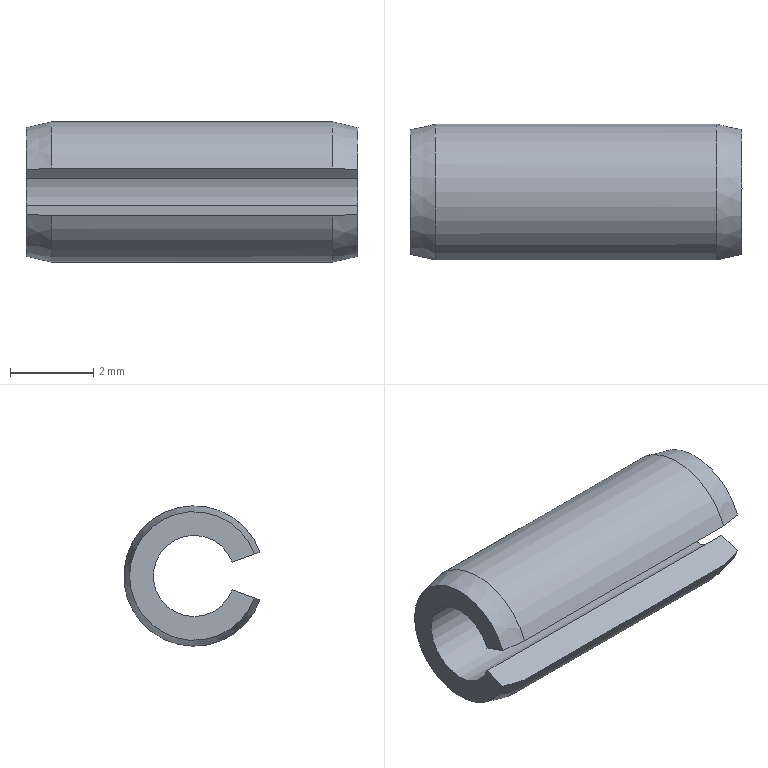Part | NX | features solid 2 | 1 solid | 8 faces | box 7.995 x 3.276 x 3.378 mm | volume 41.565 mm3 | plane 4 | cylinder 2 | cone 2 | commonest cylinder face diameters 1.956 x1 3.378 x1
STEP:
#1=CARTESIAN_POINT('',(282.619,2079.482,26.517));
#2=VERTEX_POINT('',#1);
#3=CARTESIAN_POINT('',(282.619,2079.482,27.673));
#4=VERTEX_POINT('',#3);
#5=CARTESIAN_POINT('',(282.619,2081.069,27.095));
#6=DIRECTION('',(1.,0.,-0.000000164));
#7=DIRECTION('',(-0.000000056,-0.9397,-0.342));
#8=AXIS2_PLACEMENT_3D('',#5,#6,#7);
#9=CIRCLE('',#8,1.689);
#10=EDGE_CURVE('',#2,#4,#9,.T.);
#11=ORIENTED_EDGE('',*,*,#10,.T.);
#12=CARTESIAN_POINT('',(289.395,2079.482,27.673));
#13=VERTEX_POINT('',#12);
#14=CARTESIAN_POINT('',(282.619,2079.482,27.673));
#15=DIRECTION('',(1.,0.,-0.000000164));
#16=VECTOR('',#15,1000.);
#17=LINE('',#14,#16);
#18=EDGE_CURVE('',#4,#13,#17,.T.);
#19=ORIENTED_EDGE('',*,*,#18,.T.);
#20=CARTESIAN_POINT('',(289.395,2081.069,25.406));
#21=VERTEX_POINT('',#20);
#22=CARTESIAN_POINT('',(289.395,2081.069,27.095));
#23=DIRECTION('',(1.,0.,-0.000000164));
#24=DIRECTION('',(-0.000000164,0.,-1.));
#25=AXIS2_PLACEMENT_3D('',#22,#23,#24);
#26=CIRCLE('',#25,1.689);
#27=EDGE_CURVE('',#21,#13,#26,.T.);
#28=ORIENTED_EDGE('',*,*,#27,.F.);
#29=CARTESIAN_POINT('',(289.395,2079.482,26.517));
#30=VERTEX_POINT('',#29);
#31=CARTESIAN_POINT('',(289.395,2081.069,27.095));
#32=DIRECTION('',(1.,0.,-0.000000164));
#33=DIRECTION('',(-0.000000056,-0.9397,-0.342));
#34=AXIS2_PLACEMENT_3D('',#31,#32,#33);
#35=CIRCLE('',#34,1.689);
#36=EDGE_CURVE('',#30,#21,#35,.T.);
#37=ORIENTED_EDGE('',*,*,#36,.F.);
#38=CARTESIAN_POINT('',(289.395,2079.482,26.517));
#39=DIRECTION('',(-1.,0.,0.000000164));
#40=VECTOR('',#39,1000.);
#41=LINE('',#38,#40);
#42=EDGE_CURVE('',#30,#2,#41,.T.);
#43=ORIENTED_EDGE('',*,*,#42,.T.);
#44=EDGE_LOOP('',(#11,#19,#28,#37,#43));
#45=FACE_BOUND('',#44,.T.);
#46=CARTESIAN_POINT('',(288.284,2081.069,27.095));
#47=DIRECTION('',(-1.,0.,0.000000164));
#48=DIRECTION('',(0.000000164,0.,1.));
#49=AXIS2_PLACEMENT_3D('',#46,#47,#48);
#50=CYLINDRICAL_SURFACE('',#49,1.689);
#51=ADVANCED_FACE('',(#45),#50,.T.);
#52=CARTESIAN_POINT('',(282.009,2079.613,26.565));
#53=VERTEX_POINT('',#52);
#54=CARTESIAN_POINT('',(282.009,2079.613,26.565));
#55=DIRECTION('',(0.9747,-0.2099,-0.0764));
#56=VECTOR('',#55,1000.);
#57=LINE('',#54,#56);
#58=EDGE_CURVE('',#53,#2,#57,.T.);
#59=ORIENTED_EDGE('',*,*,#58,.T.);
#60=ORIENTED_EDGE('',*,*,#42,.F.);
#61=CARTESIAN_POINT('',(290.004,2079.613,26.565));
#62=VERTEX_POINT('',#61);
#63=CARTESIAN_POINT('',(289.395,2079.482,26.517));
#64=DIRECTION('',(0.9747,0.2099,0.0764));
#65=VECTOR('',#64,1000.);
#66=LINE('',#63,#65);
#67=EDGE_CURVE('',#30,#62,#66,.T.);
#68=ORIENTED_EDGE('',*,*,#67,.T.);
#69=CARTESIAN_POINT('',(290.004,2080.15,26.761));
#70=VERTEX_POINT('',#69);
#71=CARTESIAN_POINT('',(290.004,2080.15,26.761));
#72=DIRECTION('',(-0.000000056,-0.9397,-0.342));
#73=VECTOR('',#72,1000.);
#74=LINE('',#71,#73);
#75=EDGE_CURVE('',#70,#62,#74,.T.);
#76=ORIENTED_EDGE('',*,*,#75,.F.);
#77=CARTESIAN_POINT('',(282.009,2080.15,26.761));
#78=VERTEX_POINT('',#77);
#79=CARTESIAN_POINT('',(282.009,2080.15,26.761));
#80=DIRECTION('',(1.,0.,-0.000000164));
#81=VECTOR('',#80,1000.);
#82=LINE('',#79,#81);
#83=EDGE_CURVE('',#78,#70,#82,.T.);
#84=ORIENTED_EDGE('',*,*,#83,.F.);
#85=CARTESIAN_POINT('',(282.009,2079.613,26.565));
#86=DIRECTION('',(0.000000056,0.9397,0.342));
#87=VECTOR('',#86,1000.);
#88=LINE('',#85,#87);
#89=EDGE_CURVE('',#53,#78,#88,.T.);
#90=ORIENTED_EDGE('',*,*,#89,.F.);
#91=EDGE_LOOP('',(#59,#60,#68,#76,#84,#90));
#92=FACE_BOUND('',#91,.T.);
#93=CARTESIAN_POINT('',(288.284,2080.15,26.761));
#94=DIRECTION('',(-0.000000154,0.342,-0.9397));
#95=DIRECTION('',(0.000000056,0.9397,0.342));
#96=AXIS2_PLACEMENT_3D('',#93,#94,#95);
#97=PLANE('',#96);
#98=ADVANCED_FACE('',(#92),#97,.F.);
#99=CARTESIAN_POINT('',(282.009,2079.613,27.625));
#100=VERTEX_POINT('',#99);
#101=CARTESIAN_POINT('',(282.009,2081.069,27.095));
#102=DIRECTION('',(1.,0.,-0.000000164));
#103=DIRECTION('',(-0.000000056,-0.9397,-0.342));
#104=AXIS2_PLACEMENT_3D('',#101,#102,#103);
#105=CIRCLE('',#104,1.549);
#106=EDGE_CURVE('',#53,#100,#105,.T.);
#107=ORIENTED_EDGE('',*,*,#106,.F.);
#108=ORIENTED_EDGE('',*,*,#89,.T.);
#109=CARTESIAN_POINT('',(282.009,2081.069,26.117));
#110=VERTEX_POINT('',#109);
#111=CARTESIAN_POINT('',(282.009,2081.069,27.095));
#112=DIRECTION('',(1.,0.,-0.000000164));
#113=DIRECTION('',(-0.000000056,-0.9397,-0.342));
#114=AXIS2_PLACEMENT_3D('',#111,#112,#113);
#115=CIRCLE('',#114,0.9779);
#116=EDGE_CURVE('',#78,#110,#115,.T.);
#117=ORIENTED_EDGE('',*,*,#116,.T.);
#118=CARTESIAN_POINT('',(282.009,2080.15,27.429));
#119=VERTEX_POINT('',#118);
#120=CARTESIAN_POINT('',(282.009,2081.069,27.095));
#121=DIRECTION('',(1.,0.,-0.000000164));
#122=DIRECTION('',(-0.000000164,0.,-1.));
#123=AXIS2_PLACEMENT_3D('',#120,#121,#122);
#124=CIRCLE('',#123,0.9779);
#125=EDGE_CURVE('',#110,#119,#124,.T.);
#126=ORIENTED_EDGE('',*,*,#125,.T.);
#127=CARTESIAN_POINT('',(282.009,2080.15,27.429));
#128=DIRECTION('',(0.000000056,-0.9397,0.342));
#129=VECTOR('',#128,1000.);
#130=LINE('',#127,#129);
#131=EDGE_CURVE('',#119,#100,#130,.T.);
#132=ORIENTED_EDGE('',*,*,#131,.T.);
#133=EDGE_LOOP('',(#107,#108,#117,#126,#132));
#134=FACE_BOUND('',#133,.T.);
#135=CARTESIAN_POINT('',(282.009,2081.069,27.095));
#136=DIRECTION('',(1.,0.,-0.000000164));
#137=DIRECTION('',(-0.000000164,0.,-1.));
#138=AXIS2_PLACEMENT_3D('',#135,#136,#137);
#139=PLANE('',#138);
#140=ADVANCED_FACE('',(#134),#139,.F.);
#141=CARTESIAN_POINT('',(282.619,2079.482,27.673));
#142=DIRECTION('',(-0.9747,0.2099,-0.0764));
#143=VECTOR('',#142,1000.);
#144=LINE('',#141,#143);
#145=EDGE_CURVE('',#4,#100,#144,.T.);
#146=ORIENTED_EDGE('',*,*,#145,.T.);
#147=ORIENTED_EDGE('',*,*,#131,.F.);
#148=CARTESIAN_POINT('',(290.004,2080.15,27.429));
#149=VERTEX_POINT('',#148);
#150=CARTESIAN_POINT('',(290.004,2080.15,27.429));
#151=DIRECTION('',(-1.,0.,0.000000164));
#152=VECTOR('',#151,1000.);
#153=LINE('',#150,#152);
#154=EDGE_CURVE('',#149,#119,#153,.T.);
#155=ORIENTED_EDGE('',*,*,#154,.F.);
#156=CARTESIAN_POINT('',(290.004,2079.613,27.625));
#157=VERTEX_POINT('',#156);
#158=CARTESIAN_POINT('',(290.004,2079.613,27.625));
#159=DIRECTION('',(-0.000000056,0.9397,-0.342));
#160=VECTOR('',#159,1000.);
#161=LINE('',#158,#160);
#162=EDGE_CURVE('',#157,#149,#161,.T.);
#163=ORIENTED_EDGE('',*,*,#162,.F.);
#164=CARTESIAN_POINT('',(290.004,2079.613,27.625));
#165=DIRECTION('',(-0.9747,-0.2099,0.0764));
#166=VECTOR('',#165,1000.);
#167=LINE('',#164,#166);
#168=EDGE_CURVE('',#157,#13,#167,.T.);
#169=ORIENTED_EDGE('',*,*,#168,.T.);
#170=ORIENTED_EDGE('',*,*,#18,.F.);
#171=EDGE_LOOP('',(#146,#147,#155,#163,#169,#170));
#172=FACE_BOUND('',#171,.T.);
#173=CARTESIAN_POINT('',(288.284,2079.482,27.673));
#174=DIRECTION('',(0.000000154,0.342,0.9397));
#175=DIRECTION('',(0.000000056,-0.9397,0.342));
#176=AXIS2_PLACEMENT_3D('',#173,#174,#175);
#177=PLANE('',#176);
#178=ADVANCED_FACE('',(#172),#177,.F.);
#179=ORIENTED_EDGE('',*,*,#36,.T.);
#180=ORIENTED_EDGE('',*,*,#27,.T.);
#181=ORIENTED_EDGE('',*,*,#168,.F.);
#182=CARTESIAN_POINT('',(290.004,2081.069,25.546));
#183=VERTEX_POINT('',#182);
#184=CARTESIAN_POINT('',(290.004,2081.069,27.095));
#185=DIRECTION('',(1.,0.,-0.000000164));
#186=DIRECTION('',(-0.000000164,0.,-1.));
#187=AXIS2_PLACEMENT_3D('',#184,#185,#186);
#188=CIRCLE('',#187,1.549);
#189=EDGE_CURVE('',#183,#157,#188,.T.);
#190=ORIENTED_EDGE('',*,*,#189,.F.);
#191=CARTESIAN_POINT('',(290.004,2081.069,27.095));
#192=DIRECTION('',(1.,0.,-0.000000164));
#193=DIRECTION('',(-0.000000056,-0.9397,-0.342));
#194=AXIS2_PLACEMENT_3D('',#191,#192,#193);
#195=CIRCLE('',#194,1.549);
#196=EDGE_CURVE('',#62,#183,#195,.T.);
#197=ORIENTED_EDGE('',*,*,#196,.F.);
#198=ORIENTED_EDGE('',*,*,#67,.F.);
#199=EDGE_LOOP('',(#179,#180,#181,#190,#197,#198));
#200=FACE_BOUND('',#199,.T.);
#201=CARTESIAN_POINT('',(289.699,2081.069,27.095));
#202=DIRECTION('',(-1.,0.,0.000000164));
#203=DIRECTION('',(0.000000164,0.,1.));
#204=AXIS2_PLACEMENT_3D('',#201,#202,#203);
#205=CONICAL_SURFACE('',#204,1.619,0.2253);
#206=ADVANCED_FACE('',(#200),#205,.T.);
#207=ORIENTED_EDGE('',*,*,#196,.T.);
#208=ORIENTED_EDGE('',*,*,#189,.T.);
#209=ORIENTED_EDGE('',*,*,#162,.T.);
#210=CARTESIAN_POINT('',(290.004,2081.069,26.117));
#211=VERTEX_POINT('',#210);
#212=CARTESIAN_POINT('',(290.004,2081.069,27.095));
#213=DIRECTION('',(-1.,0.,0.000000164));
#214=DIRECTION('',(0.000000056,-0.9397,0.342));
#215=AXIS2_PLACEMENT_3D('',#212,#213,#214);
#216=CIRCLE('',#215,0.9779);
#217=EDGE_CURVE('',#149,#211,#216,.T.);
#218=ORIENTED_EDGE('',*,*,#217,.T.);
#219=CARTESIAN_POINT('',(290.004,2081.069,27.095));
#220=DIRECTION('',(-1.,0.,0.000000164));
#221=DIRECTION('',(-0.000000164,0.,-1.));
#222=AXIS2_PLACEMENT_3D('',#219,#220,#221);
#223=CIRCLE('',#222,0.9779);
#224=EDGE_CURVE('',#211,#70,#223,.T.);
#225=ORIENTED_EDGE('',*,*,#224,.T.);
#226=ORIENTED_EDGE('',*,*,#75,.T.);
#227=EDGE_LOOP('',(#207,#208,#209,#218,#225,#226));
#228=FACE_BOUND('',#227,.T.);
#229=CARTESIAN_POINT('',(290.004,2081.069,27.095));
#230=DIRECTION('',(1.,0.,-0.000000164));
#231=DIRECTION('',(-0.000000164,0.,-1.));
#232=AXIS2_PLACEMENT_3D('',#229,#230,#231);
#233=PLANE('',#232);
#234=ADVANCED_FACE('',(#228),#233,.T.);
#235=ORIENTED_EDGE('',*,*,#116,.F.);
#236=ORIENTED_EDGE('',*,*,#83,.T.);
#237=ORIENTED_EDGE('',*,*,#224,.F.);
#238=ORIENTED_EDGE('',*,*,#217,.F.);
#239=ORIENTED_EDGE('',*,*,#154,.T.);
#240=ORIENTED_EDGE('',*,*,#125,.F.);
#241=EDGE_LOOP('',(#235,#236,#237,#238,#239,#240));
#242=FACE_BOUND('',#241,.T.);
#243=CARTESIAN_POINT('',(288.284,2081.069,27.095));
#244=DIRECTION('',(-1.,0.,0.000000164));
#245=DIRECTION('',(0.000000164,0.,1.));
#246=AXIS2_PLACEMENT_3D('',#243,#244,#245);
#247=CYLINDRICAL_SURFACE('',#246,0.9779);
#248=ADVANCED_FACE('',(#242),#247,.F.);
#249=ORIENTED_EDGE('',*,*,#106,.T.);
#250=ORIENTED_EDGE('',*,*,#145,.F.);
#251=ORIENTED_EDGE('',*,*,#10,.F.);
#252=ORIENTED_EDGE('',*,*,#58,.F.);
#253=EDGE_LOOP('',(#249,#250,#251,#252));
#254=FACE_BOUND('',#253,.T.);
#255=CARTESIAN_POINT('',(282.314,2081.069,27.095));
#256=DIRECTION('',(1.,0.,-0.000000164));
#257=DIRECTION('',(-0.000000164,0.,-1.));
#258=AXIS2_PLACEMENT_3D('',#255,#256,#257);
#259=CONICAL_SURFACE('',#258,1.619,0.2253);
#260=ADVANCED_FACE('',(#254),#259,.T.);
#261=CLOSED_SHELL('',(#51,#98,#140,#178,#206,#234,#248,#260));
#262=MANIFOLD_SOLID_BREP('',#261);
#263=(LENGTH_UNIT()NAMED_UNIT(*)SI_UNIT(.MILLI.,.METRE.));
#264=UNCERTAINTY_MEASURE_WITH_UNIT(LENGTH_MEASURE(0.00001),#263,'','');
#265=(NAMED_UNIT(*)PLANE_ANGLE_UNIT()SI_UNIT($,.RADIAN.));
#266=(NAMED_UNIT(*)SI_UNIT($,.STERADIAN.)SOLID_ANGLE_UNIT());
#267=(GEOMETRIC_REPRESENTATION_CONTEXT(3)GLOBAL_UNCERTAINTY_ASSIGNED_CONTEXT((#264))GLOBAL_UNIT_ASSIGNED_CONTEXT((#263,#265,#266))REPRESENTATION_CONTEXT('',''));
#268=ADVANCED_BREP_SHAPE_REPRESENTATION('',(#262),#267);